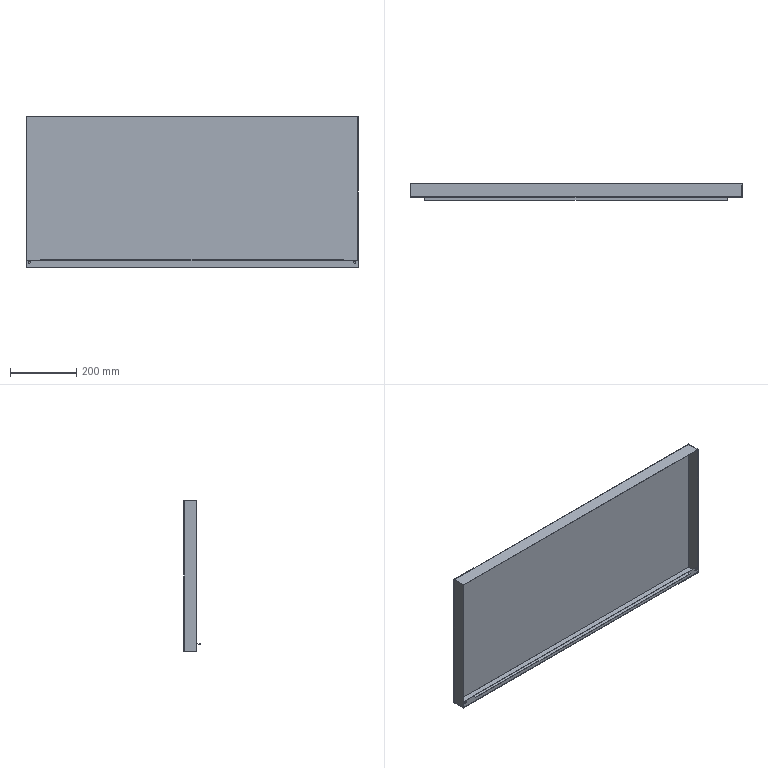Part | SolidWorks | features ICE 4, ExtruThin 1 | 1 solid | 23 faces | box 1002 x 50 x 455 mm | volume 600406 mm3 | plane 19 | cylinder 4 | commonest cylinder face diameters 5.5 x4
STEP:
#1=CARTESIAN_POINT('',(-491.,-39.,17.75));
#2=VERTEX_POINT('',#1);
#3=CARTESIAN_POINT('',(-491.,-39.,12.25));
#4=VERTEX_POINT('',#3);
#5=CARTESIAN_POINT('',(-491.,-39.,15.));
#6=DIRECTION('',(0.,-1.,0.));
#7=DIRECTION('',(0.,0.,-1.));
#8=AXIS2_PLACEMENT_3D('',#5,#6,#7);
#9=CIRCLE('',#8,2.75);
#10=EDGE_CURVE('',#2,#4,#9,.T.);
#11=ORIENTED_EDGE('',*,*,#10,.F.);
#12=CARTESIAN_POINT('',(-491.,-40.,17.75));
#13=VERTEX_POINT('',#12);
#14=CARTESIAN_POINT('',(-491.,-30.,17.75));
#15=DIRECTION('',(0.,-1.,0.));
#16=VECTOR('',#15,1000.);
#17=LINE('',#14,#16);
#18=EDGE_CURVE('',#2,#13,#17,.T.);
#19=ORIENTED_EDGE('',*,*,#18,.T.);
#20=CARTESIAN_POINT('',(-491.,-40.,12.25));
#21=VERTEX_POINT('',#20);
#22=CARTESIAN_POINT('',(-491.,-40.,15.));
#23=DIRECTION('',(0.,-1.,0.));
#24=DIRECTION('',(0.,0.,1.));
#25=AXIS2_PLACEMENT_3D('',#22,#23,#24);
#26=CIRCLE('',#25,2.75);
#27=EDGE_CURVE('',#13,#21,#26,.T.);
#28=ORIENTED_EDGE('',*,*,#27,.T.);
#29=CARTESIAN_POINT('',(-491.,-30.,12.25));
#30=DIRECTION('',(0.,-1.,0.));
#31=VECTOR('',#30,1000.);
#32=LINE('',#29,#31);
#33=EDGE_CURVE('',#4,#21,#32,.T.);
#34=ORIENTED_EDGE('',*,*,#33,.F.);
#35=EDGE_LOOP('',(#11,#19,#28,#34));
#36=FACE_OUTER_BOUND('',#35,.T.);
#37=CARTESIAN_POINT('',(-491.,-30.,15.));
#38=DIRECTION('',(0.,-1.,0.));
#39=DIRECTION('',(0.,0.,-1.));
#40=AXIS2_PLACEMENT_3D('',#37,#38,#39);
#41=CYLINDRICAL_SURFACE('',#40,2.75);
#42=ADVANCED_FACE('',(#36),#41,.F.);
#43=CARTESIAN_POINT('',(491.,-39.,17.75));
#44=VERTEX_POINT('',#43);
#45=CARTESIAN_POINT('',(491.,-39.,12.25));
#46=VERTEX_POINT('',#45);
#47=CARTESIAN_POINT('',(491.,-39.,15.));
#48=DIRECTION('',(0.,-1.,0.));
#49=DIRECTION('',(0.,0.,-1.));
#50=AXIS2_PLACEMENT_3D('',#47,#48,#49);
#51=CIRCLE('',#50,2.75);
#52=EDGE_CURVE('',#44,#46,#51,.T.);
#53=ORIENTED_EDGE('',*,*,#52,.F.);
#54=CARTESIAN_POINT('',(491.,-40.,17.75));
#55=VERTEX_POINT('',#54);
#56=CARTESIAN_POINT('',(491.,-30.,17.75));
#57=DIRECTION('',(0.,-1.,0.));
#58=VECTOR('',#57,1000.);
#59=LINE('',#56,#58);
#60=EDGE_CURVE('',#44,#55,#59,.T.);
#61=ORIENTED_EDGE('',*,*,#60,.T.);
#62=CARTESIAN_POINT('',(491.,-40.,12.25));
#63=VERTEX_POINT('',#62);
#64=CARTESIAN_POINT('',(491.,-40.,15.));
#65=DIRECTION('',(0.,-1.,0.));
#66=DIRECTION('',(0.,0.,-1.));
#67=AXIS2_PLACEMENT_3D('',#64,#65,#66);
#68=CIRCLE('',#67,2.75);
#69=EDGE_CURVE('',#55,#63,#68,.T.);
#70=ORIENTED_EDGE('',*,*,#69,.T.);
#71=CARTESIAN_POINT('',(491.,-30.,12.25));
#72=DIRECTION('',(0.,-1.,0.));
#73=VECTOR('',#72,1000.);
#74=LINE('',#71,#73);
#75=EDGE_CURVE('',#46,#63,#74,.T.);
#76=ORIENTED_EDGE('',*,*,#75,.F.);
#77=EDGE_LOOP('',(#53,#61,#70,#76));
#78=FACE_OUTER_BOUND('',#77,.T.);
#79=CARTESIAN_POINT('',(491.,-30.,15.));
#80=DIRECTION('',(0.,-1.,0.));
#81=DIRECTION('',(0.,0.,-1.));
#82=AXIS2_PLACEMENT_3D('',#79,#80,#81);
#83=CYLINDRICAL_SURFACE('',#82,2.75);
#84=ADVANCED_FACE('',(#78),#83,.F.);
#85=CARTESIAN_POINT('',(457.,-39.,23.));
#86=VERTEX_POINT('',#85);
#87=CARTESIAN_POINT('',(-457.,-39.,23.));
#88=VERTEX_POINT('',#87);
#89=CARTESIAN_POINT('',(500.,-39.,23.));
#90=DIRECTION('',(-1.,0.,0.));
#91=VECTOR('',#90,1000.);
#92=LINE('',#89,#91);
#93=EDGE_CURVE('',#86,#88,#92,.T.);
#94=ORIENTED_EDGE('',*,*,#93,.T.);
#95=CARTESIAN_POINT('',(-457.,-50.,23.));
#96=VERTEX_POINT('',#95);
#97=CARTESIAN_POINT('',(-457.,-30.,23.));
#98=DIRECTION('',(0.,-1.,0.));
#99=VECTOR('',#98,1000.);
#100=LINE('',#97,#99);
#101=EDGE_CURVE('',#88,#96,#100,.T.);
#102=ORIENTED_EDGE('',*,*,#101,.T.);
#103=CARTESIAN_POINT('',(457.,-50.,23.));
#104=VERTEX_POINT('',#103);
#105=CARTESIAN_POINT('',(500.,-50.,23.));
#106=DIRECTION('',(-1.,0.,0.));
#107=VECTOR('',#106,1000.);
#108=LINE('',#105,#107);
#109=EDGE_CURVE('',#104,#96,#108,.T.);
#110=ORIENTED_EDGE('',*,*,#109,.F.);
#111=CARTESIAN_POINT('',(457.,-30.,23.));
#112=DIRECTION('',(0.,-1.,0.));
#113=VECTOR('',#112,1000.);
#114=LINE('',#111,#113);
#115=EDGE_CURVE('',#86,#104,#114,.T.);
#116=ORIENTED_EDGE('',*,*,#115,.F.);
#117=EDGE_LOOP('',(#94,#102,#110,#116));
#118=FACE_OUTER_BOUND('',#117,.T.);
#119=CARTESIAN_POINT('',(500.,-40.,23.));
#120=DIRECTION('',(0.,0.,-1.));
#121=DIRECTION('',(-1.,0.,0.));
#122=AXIS2_PLACEMENT_3D('',#119,#120,#121);
#123=PLANE('',#122);
#124=ADVANCED_FACE('',(#118),#123,.F.);
#125=CARTESIAN_POINT('',(-457.,-50.,22.));
#126=VERTEX_POINT('',#125);
#127=CARTESIAN_POINT('',(-457.,-50.,22.));
#128=DIRECTION('',(0.,0.,1.));
#129=VECTOR('',#128,1000.);
#130=LINE('',#127,#129);
#131=EDGE_CURVE('',#126,#96,#130,.T.);
#132=ORIENTED_EDGE('',*,*,#131,.F.);
#133=CARTESIAN_POINT('',(457.,-50.,22.));
#134=VERTEX_POINT('',#133);
#135=CARTESIAN_POINT('',(500.,-50.,22.));
#136=DIRECTION('',(-1.,0.,0.));
#137=VECTOR('',#136,1000.);
#138=LINE('',#135,#137);
#139=EDGE_CURVE('',#134,#126,#138,.T.);
#140=ORIENTED_EDGE('',*,*,#139,.F.);
#141=CARTESIAN_POINT('',(457.,-50.,23.));
#142=DIRECTION('',(0.,0.,-1.));
#143=VECTOR('',#142,1000.);
#144=LINE('',#141,#143);
#145=EDGE_CURVE('',#104,#134,#144,.T.);
#146=ORIENTED_EDGE('',*,*,#145,.F.);
#147=ORIENTED_EDGE('',*,*,#109,.T.);
#148=EDGE_LOOP('',(#132,#140,#146,#147));
#149=FACE_OUTER_BOUND('',#148,.T.);
#150=CARTESIAN_POINT('',(500.,-50.,22.));
#151=DIRECTION('',(0.,-1.,0.));
#152=DIRECTION('',(0.,0.,-1.));
#153=AXIS2_PLACEMENT_3D('',#150,#151,#152);
#154=PLANE('',#153);
#155=ADVANCED_FACE('',(#149),#154,.T.);
#156=CARTESIAN_POINT('',(-457.,-40.,22.));
#157=VERTEX_POINT('',#156);
#158=CARTESIAN_POINT('',(-457.,-30.,22.));
#159=DIRECTION('',(0.,-1.,0.));
#160=VECTOR('',#159,1000.);
#161=LINE('',#158,#160);
#162=EDGE_CURVE('',#157,#126,#161,.T.);
#163=ORIENTED_EDGE('',*,*,#162,.F.);
#164=CARTESIAN_POINT('',(457.,-40.,22.));
#165=VERTEX_POINT('',#164);
#166=CARTESIAN_POINT('',(500.,-40.,22.));
#167=DIRECTION('',(-1.,0.,0.));
#168=VECTOR('',#167,1000.);
#169=LINE('',#166,#168);
#170=EDGE_CURVE('',#165,#157,#169,.T.);
#171=ORIENTED_EDGE('',*,*,#170,.F.);
#172=CARTESIAN_POINT('',(457.,-30.,22.));
#173=DIRECTION('',(0.,-1.,0.));
#174=VECTOR('',#173,1000.);
#175=LINE('',#172,#174);
#176=EDGE_CURVE('',#165,#134,#175,.T.);
#177=ORIENTED_EDGE('',*,*,#176,.T.);
#178=ORIENTED_EDGE('',*,*,#139,.T.);
#179=EDGE_LOOP('',(#163,#171,#177,#178));
#180=FACE_OUTER_BOUND('',#179,.T.);
#181=CARTESIAN_POINT('',(500.,-40.,22.));
#182=DIRECTION('',(0.,0.,-1.));
#183=DIRECTION('',(-1.,0.,0.));
#184=AXIS2_PLACEMENT_3D('',#181,#182,#183);
#185=PLANE('',#184);
#186=ADVANCED_FACE('',(#180),#185,.T.);
#187=CARTESIAN_POINT('',(501.,-40.,0.));
#188=VERTEX_POINT('',#187);
#189=CARTESIAN_POINT('',(-501.,-40.,0.));
#190=VERTEX_POINT('',#189);
#191=CARTESIAN_POINT('',(500.,-40.,0.));
#192=DIRECTION('',(-1.,0.,0.));
#193=VECTOR('',#192,1000.);
#194=LINE('',#191,#193);
#195=EDGE_CURVE('',#188,#190,#194,.T.);
#196=ORIENTED_EDGE('',*,*,#195,.T.);
#197=CARTESIAN_POINT('',(-501.,0.,0.));
#198=VERTEX_POINT('',#197);
#199=CARTESIAN_POINT('',(-501.,-40.,0.));
#200=DIRECTION('',(0.,-1.,0.));
#201=VECTOR('',#200,1000.);
#202=LINE('',#199,#201);
#203=EDGE_CURVE('',#198,#190,#202,.T.);
#204=ORIENTED_EDGE('',*,*,#203,.F.);
#205=CARTESIAN_POINT('',(501.,0.,0.));
#206=VERTEX_POINT('',#205);
#207=CARTESIAN_POINT('',(500.,0.,0.));
#208=DIRECTION('',(-1.,0.,0.));
#209=VECTOR('',#208,1000.);
#210=LINE('',#207,#209);
#211=EDGE_CURVE('',#206,#198,#210,.T.);
#212=ORIENTED_EDGE('',*,*,#211,.F.);
#213=CARTESIAN_POINT('',(501.,0.,0.));
#214=DIRECTION('',(0.,1.,0.));
#215=VECTOR('',#214,1000.);
#216=LINE('',#213,#215);
#217=EDGE_CURVE('',#188,#206,#216,.T.);
#218=ORIENTED_EDGE('',*,*,#217,.F.);
#219=EDGE_LOOP('',(#196,#204,#212,#218));
#220=FACE_OUTER_BOUND('',#219,.T.);
#221=CARTESIAN_POINT('',(500.,0.,0.));
#222=DIRECTION('',(0.,0.,-1.));
#223=DIRECTION('',(-1.,0.,0.));
#224=AXIS2_PLACEMENT_3D('',#221,#222,#223);
#225=PLANE('',#224);
#226=ADVANCED_FACE('',(#220),#225,.T.);
#227=ORIENTED_EDGE('',*,*,#211,.T.);
#228=CARTESIAN_POINT('',(-501.,0.,455.));
#229=VERTEX_POINT('',#228);
#230=CARTESIAN_POINT('',(-501.,0.,0.));
#231=DIRECTION('',(0.,0.,-1.));
#232=VECTOR('',#231,1000.);
#233=LINE('',#230,#232);
#234=EDGE_CURVE('',#229,#198,#233,.T.);
#235=ORIENTED_EDGE('',*,*,#234,.F.);
#236=CARTESIAN_POINT('',(501.,0.,455.));
#237=VERTEX_POINT('',#236);
#238=CARTESIAN_POINT('',(500.,0.,455.));
#239=DIRECTION('',(-1.,0.,0.));
#240=VECTOR('',#239,1000.);
#241=LINE('',#238,#240);
#242=EDGE_CURVE('',#237,#229,#241,.T.);
#243=ORIENTED_EDGE('',*,*,#242,.F.);
#244=CARTESIAN_POINT('',(501.,0.,455.));
#245=DIRECTION('',(0.,0.,1.));
#246=VECTOR('',#245,1000.);
#247=LINE('',#244,#246);
#248=EDGE_CURVE('',#206,#237,#247,.T.);
#249=ORIENTED_EDGE('',*,*,#248,.F.);
#250=EDGE_LOOP('',(#227,#235,#243,#249));
#251=FACE_OUTER_BOUND('',#250,.T.);
#252=CARTESIAN_POINT('',(500.,0.,0.));
#253=DIRECTION('',(0.,1.,0.));
#254=DIRECTION('',(0.,0.,1.));
#255=AXIS2_PLACEMENT_3D('',#252,#253,#254);
#256=PLANE('',#255);
#257=ADVANCED_FACE('',(#251),#256,.T.);
#258=ORIENTED_EDGE('',*,*,#242,.T.);
#259=CARTESIAN_POINT('',(-501.,-40.,455.));
#260=VERTEX_POINT('',#259);
#261=CARTESIAN_POINT('',(-501.,0.,455.));
#262=DIRECTION('',(0.,1.,0.));
#263=VECTOR('',#262,1000.);
#264=LINE('',#261,#263);
#265=EDGE_CURVE('',#260,#229,#264,.T.);
#266=ORIENTED_EDGE('',*,*,#265,.F.);
#267=CARTESIAN_POINT('',(501.,-40.,455.));
#268=VERTEX_POINT('',#267);
#269=CARTESIAN_POINT('',(500.,-40.,455.));
#270=DIRECTION('',(-1.,0.,0.));
#271=VECTOR('',#270,1000.);
#272=LINE('',#269,#271);
#273=EDGE_CURVE('',#268,#260,#272,.T.);
#274=ORIENTED_EDGE('',*,*,#273,.F.);
#275=CARTESIAN_POINT('',(501.,-40.,455.));
#276=DIRECTION('',(0.,-1.,0.));
#277=VECTOR('',#276,1000.);
#278=LINE('',#275,#277);
#279=EDGE_CURVE('',#237,#268,#278,.T.);
#280=ORIENTED_EDGE('',*,*,#279,.F.);
#281=EDGE_LOOP('',(#258,#266,#274,#280));
#282=FACE_OUTER_BOUND('',#281,.T.);
#283=CARTESIAN_POINT('',(500.,0.,455.));
#284=DIRECTION('',(0.,0.,1.));
#285=DIRECTION('',(1.,0.,0.));
#286=AXIS2_PLACEMENT_3D('',#283,#284,#285);
#287=PLANE('',#286);
#288=ADVANCED_FACE('',(#282),#287,.T.);
#289=CARTESIAN_POINT('',(-491.,-40.,15.));
#290=DIRECTION('',(0.,-1.,0.));
#291=DIRECTION('',(0.,0.,1.));
#292=AXIS2_PLACEMENT_3D('',#289,#290,#291);
#293=CIRCLE('',#292,2.75);
#294=EDGE_CURVE('',#21,#13,#293,.T.);
#295=ORIENTED_EDGE('',*,*,#294,.F.);
#296=ORIENTED_EDGE('',*,*,#27,.F.);
#297=EDGE_LOOP('',(#295,#296));
#298=FACE_BOUND('',#297,.T.);
#299=CARTESIAN_POINT('',(491.,-40.,15.));
#300=DIRECTION('',(0.,-1.,0.));
#301=DIRECTION('',(0.,0.,-1.));
#302=AXIS2_PLACEMENT_3D('',#299,#300,#301);
#303=CIRCLE('',#302,2.75);
#304=EDGE_CURVE('',#63,#55,#303,.T.);
#305=ORIENTED_EDGE('',*,*,#304,.F.);
#306=ORIENTED_EDGE('',*,*,#69,.F.);
#307=EDGE_LOOP('',(#305,#306));
#308=FACE_BOUND('',#307,.T.);
#309=CARTESIAN_POINT('',(500.,-40.,22.));
#310=VERTEX_POINT('',#309);
#311=CARTESIAN_POINT('',(500.,-40.,22.));
#312=DIRECTION('',(-1.,0.,0.));
#313=VECTOR('',#312,1000.);
#314=LINE('',#311,#313);
#315=EDGE_CURVE('',#310,#165,#314,.T.);
#316=ORIENTED_EDGE('',*,*,#315,.T.);
#317=ORIENTED_EDGE('',*,*,#170,.T.);
#318=CARTESIAN_POINT('',(-500.,-40.,22.));
#319=VERTEX_POINT('',#318);
#320=CARTESIAN_POINT('',(500.,-40.,22.));
#321=DIRECTION('',(1.,0.,0.));
#322=VECTOR('',#321,1000.);
#323=LINE('',#320,#322);
#324=EDGE_CURVE('',#319,#157,#323,.T.);
#325=ORIENTED_EDGE('',*,*,#324,.F.);
#326=CARTESIAN_POINT('',(-500.,-40.,454.));
#327=VERTEX_POINT('',#326);
#328=CARTESIAN_POINT('',(-500.,-40.,455.));
#329=DIRECTION('',(0.,0.,1.));
#330=VECTOR('',#329,1000.);
#331=LINE('',#328,#330);
#332=EDGE_CURVE('',#319,#327,#331,.T.);
#333=ORIENTED_EDGE('',*,*,#332,.T.);
#334=CARTESIAN_POINT('',(500.,-40.,454.));
#335=VERTEX_POINT('',#334);
#336=CARTESIAN_POINT('',(500.,-40.,454.));
#337=DIRECTION('',(-1.,0.,0.));
#338=VECTOR('',#337,1000.);
#339=LINE('',#336,#338);
#340=EDGE_CURVE('',#335,#327,#339,.T.);
#341=ORIENTED_EDGE('',*,*,#340,.F.);
#342=CARTESIAN_POINT('',(500.,-40.,0.));
#343=DIRECTION('',(0.,0.,-1.));
#344=VECTOR('',#343,1000.);
#345=LINE('',#342,#344);
#346=EDGE_CURVE('',#335,#310,#345,.T.);
#347=ORIENTED_EDGE('',*,*,#346,.T.);
#348=EDGE_LOOP('',(#316,#317,#325,#333,#341,#347));
#349=FACE_BOUND('',#348,.T.);
#350=ORIENTED_EDGE('',*,*,#273,.T.);
#351=CARTESIAN_POINT('',(-501.,-40.,455.));
#352=DIRECTION('',(0.,0.,1.));
#353=VECTOR('',#352,1000.);
#354=LINE('',#351,#353);
#355=EDGE_CURVE('',#190,#260,#354,.T.);
#356=ORIENTED_EDGE('',*,*,#355,.F.);
#357=ORIENTED_EDGE('',*,*,#195,.F.);
#358=CARTESIAN_POINT('',(501.,-40.,0.));
#359=DIRECTION('',(0.,0.,-1.));
#360=VECTOR('',#359,1000.);
#361=LINE('',#358,#360);
#362=EDGE_CURVE('',#268,#188,#361,.T.);
#363=ORIENTED_EDGE('',*,*,#362,.F.);
#364=EDGE_LOOP('',(#350,#356,#357,#363));
#365=FACE_OUTER_BOUND('',#364,.T.);
#366=CARTESIAN_POINT('',(500.,-40.,454.));
#367=DIRECTION('',(0.,-1.,0.));
#368=DIRECTION('',(0.,0.,-1.));
#369=AXIS2_PLACEMENT_3D('',#366,#367,#368);
#370=PLANE('',#369);
#371=ADVANCED_FACE('',(#298,#308,#349,#365),#370,.T.);
#372=CARTESIAN_POINT('',(-500.,-1.,454.));
#373=VERTEX_POINT('',#372);
#374=CARTESIAN_POINT('',(-500.,0.,454.));
#375=DIRECTION('',(0.,1.,0.));
#376=VECTOR('',#375,1000.);
#377=LINE('',#374,#376);
#378=EDGE_CURVE('',#327,#373,#377,.T.);
#379=ORIENTED_EDGE('',*,*,#378,.T.);
#380=CARTESIAN_POINT('',(500.,-1.,454.));
#381=VERTEX_POINT('',#380);
#382=CARTESIAN_POINT('',(500.,-1.,454.));
#383=DIRECTION('',(-1.,0.,0.));
#384=VECTOR('',#383,1000.);
#385=LINE('',#382,#384);
#386=EDGE_CURVE('',#381,#373,#385,.T.);
#387=ORIENTED_EDGE('',*,*,#386,.F.);
#388=CARTESIAN_POINT('',(500.,0.,454.));
#389=DIRECTION('',(0.,1.,0.));
#390=VECTOR('',#389,1000.);
#391=LINE('',#388,#390);
#392=EDGE_CURVE('',#335,#381,#391,.T.);
#393=ORIENTED_EDGE('',*,*,#392,.F.);
#394=ORIENTED_EDGE('',*,*,#340,.T.);
#395=EDGE_LOOP('',(#379,#387,#393,#394));
#396=FACE_OUTER_BOUND('',#395,.T.);
#397=CARTESIAN_POINT('',(500.,0.,454.));
#398=DIRECTION('',(0.,0.,1.));
#399=DIRECTION('',(1.,0.,0.));
#400=AXIS2_PLACEMENT_3D('',#397,#398,#399);
#401=PLANE('',#400);
#402=ADVANCED_FACE('',(#396),#401,.F.);
#403=CARTESIAN_POINT('',(-500.,-1.,1.));
#404=VERTEX_POINT('',#403);
#405=CARTESIAN_POINT('',(-500.,-1.,0.));
#406=DIRECTION('',(0.,0.,-1.));
#407=VECTOR('',#406,1000.);
#408=LINE('',#405,#407);
#409=EDGE_CURVE('',#373,#404,#408,.T.);
#410=ORIENTED_EDGE('',*,*,#409,.T.);
#411=CARTESIAN_POINT('',(500.,-1.,1.));
#412=VERTEX_POINT('',#411);
#413=CARTESIAN_POINT('',(500.,-1.,1.));
#414=DIRECTION('',(-1.,0.,0.));
#415=VECTOR('',#414,1000.);
#416=LINE('',#413,#415);
#417=EDGE_CURVE('',#412,#404,#416,.T.);
#418=ORIENTED_EDGE('',*,*,#417,.F.);
#419=CARTESIAN_POINT('',(500.,-1.,0.));
#420=DIRECTION('',(0.,0.,-1.));
#421=VECTOR('',#420,1000.);
#422=LINE('',#419,#421);
#423=EDGE_CURVE('',#381,#412,#422,.T.);
#424=ORIENTED_EDGE('',*,*,#423,.F.);
#425=ORIENTED_EDGE('',*,*,#386,.T.);
#426=EDGE_LOOP('',(#410,#418,#424,#425));
#427=FACE_OUTER_BOUND('',#426,.T.);
#428=CARTESIAN_POINT('',(500.,-1.,0.));
#429=DIRECTION('',(0.,1.,0.));
#430=DIRECTION('',(0.,0.,1.));
#431=AXIS2_PLACEMENT_3D('',#428,#429,#430);
#432=PLANE('',#431);
#433=ADVANCED_FACE('',(#427),#432,.F.);
#434=CARTESIAN_POINT('',(-500.,-39.,1.));
#435=VERTEX_POINT('',#434);
#436=CARTESIAN_POINT('',(-500.,0.,1.));
#437=DIRECTION('',(0.,-1.,0.));
#438=VECTOR('',#437,1000.);
#439=LINE('',#436,#438);
#440=EDGE_CURVE('',#404,#435,#439,.T.);
#441=ORIENTED_EDGE('',*,*,#440,.T.);
#442=CARTESIAN_POINT('',(500.,-39.,1.));
#443=VERTEX_POINT('',#442);
#444=CARTESIAN_POINT('',(500.,-39.,1.));
#445=DIRECTION('',(-1.,0.,0.));
#446=VECTOR('',#445,1000.);
#447=LINE('',#444,#446);
#448=EDGE_CURVE('',#443,#435,#447,.T.);
#449=ORIENTED_EDGE('',*,*,#448,.F.);
#450=CARTESIAN_POINT('',(500.,0.,1.));
#451=DIRECTION('',(0.,-1.,0.));
#452=VECTOR('',#451,1000.);
#453=LINE('',#450,#452);
#454=EDGE_CURVE('',#412,#443,#453,.T.);
#455=ORIENTED_EDGE('',*,*,#454,.F.);
#456=ORIENTED_EDGE('',*,*,#417,.T.);
#457=EDGE_LOOP('',(#441,#449,#455,#456));
#458=FACE_OUTER_BOUND('',#457,.T.);
#459=CARTESIAN_POINT('',(500.,0.,1.));
#460=DIRECTION('',(0.,0.,-1.));
#461=DIRECTION('',(-1.,0.,0.));
#462=AXIS2_PLACEMENT_3D('',#459,#460,#461);
#463=PLANE('',#462);
#464=ADVANCED_FACE('',(#458),#463,.F.);
#465=CARTESIAN_POINT('',(-491.,-39.,15.));
#466=DIRECTION('',(0.,-1.,0.));
#467=DIRECTION('',(0.,0.,-1.));
#468=AXIS2_PLACEMENT_3D('',#465,#466,#467);
#469=CIRCLE('',#468,2.75);
#470=EDGE_CURVE('',#4,#2,#469,.T.);
#471=ORIENTED_EDGE('',*,*,#470,.T.);
#472=ORIENTED_EDGE('',*,*,#10,.T.);
#473=EDGE_LOOP('',(#471,#472));
#474=FACE_BOUND('',#473,.T.);
#475=CARTESIAN_POINT('',(491.,-39.,15.));
#476=DIRECTION('',(0.,-1.,0.));
#477=DIRECTION('',(0.,0.,-1.));
#478=AXIS2_PLACEMENT_3D('',#475,#476,#477);
#479=CIRCLE('',#478,2.75);
#480=EDGE_CURVE('',#46,#44,#479,.T.);
#481=ORIENTED_EDGE('',*,*,#480,.T.);
#482=ORIENTED_EDGE('',*,*,#52,.T.);
#483=EDGE_LOOP('',(#481,#482));
#484=FACE_BOUND('',#483,.T.);
#485=CARTESIAN_POINT('',(-500.,-39.,22.));
#486=VERTEX_POINT('',#485);
#487=CARTESIAN_POINT('',(-457.,-39.,22.));
#488=VERTEX_POINT('',#487);
#489=CARTESIAN_POINT('',(500.,-39.,22.));
#490=DIRECTION('',(1.,0.,0.));
#491=VECTOR('',#490,1000.);
#492=LINE('',#489,#491);
#493=EDGE_CURVE('',#486,#488,#492,.T.);
#494=ORIENTED_EDGE('',*,*,#493,.T.);
#495=CARTESIAN_POINT('',(-457.,-39.,0.));
#496=DIRECTION('',(0.,0.,1.));
#497=VECTOR('',#496,1000.);
#498=LINE('',#495,#497);
#499=EDGE_CURVE('',#488,#88,#498,.T.);
#500=ORIENTED_EDGE('',*,*,#499,.T.);
#501=ORIENTED_EDGE('',*,*,#93,.F.);
#502=CARTESIAN_POINT('',(457.,-39.,22.));
#503=VERTEX_POINT('',#502);
#504=CARTESIAN_POINT('',(457.,-39.,0.));
#505=DIRECTION('',(0.,0.,-1.));
#506=VECTOR('',#505,1000.);
#507=LINE('',#504,#506);
#508=EDGE_CURVE('',#86,#503,#507,.T.);
#509=ORIENTED_EDGE('',*,*,#508,.T.);
#510=CARTESIAN_POINT('',(500.,-39.,22.));
#511=VERTEX_POINT('',#510);
#512=CARTESIAN_POINT('',(500.,-39.,22.));
#513=DIRECTION('',(1.,0.,0.));
#514=VECTOR('',#513,1000.);
#515=LINE('',#512,#514);
#516=EDGE_CURVE('',#503,#511,#515,.T.);
#517=ORIENTED_EDGE('',*,*,#516,.T.);
#518=CARTESIAN_POINT('',(500.,-39.,0.));
#519=DIRECTION('',(0.,0.,1.));
#520=VECTOR('',#519,1000.);
#521=LINE('',#518,#520);
#522=EDGE_CURVE('',#443,#511,#521,.T.);
#523=ORIENTED_EDGE('',*,*,#522,.F.);
#524=ORIENTED_EDGE('',*,*,#448,.T.);
#525=CARTESIAN_POINT('',(-500.,-39.,0.));
#526=DIRECTION('',(0.,0.,1.));
#527=VECTOR('',#526,1000.);
#528=LINE('',#525,#527);
#529=EDGE_CURVE('',#435,#486,#528,.T.);
#530=ORIENTED_EDGE('',*,*,#529,.T.);
#531=EDGE_LOOP('',(#494,#500,#501,#509,#517,#523,#524,#530));
#532=FACE_OUTER_BOUND('',#531,.T.);
#533=CARTESIAN_POINT('',(500.,-39.,0.));
#534=DIRECTION('',(0.,-1.,0.));
#535=DIRECTION('',(0.,0.,-1.));
#536=AXIS2_PLACEMENT_3D('',#533,#534,#535);
#537=PLANE('',#536);
#538=ADVANCED_FACE('',(#474,#484,#532),#537,.F.);
#539=ORIENTED_EDGE('',*,*,#362,.T.);
#540=ORIENTED_EDGE('',*,*,#217,.T.);
#541=ORIENTED_EDGE('',*,*,#248,.T.);
#542=ORIENTED_EDGE('',*,*,#279,.T.);
#543=EDGE_LOOP('',(#539,#540,#541,#542));
#544=FACE_OUTER_BOUND('',#543,.T.);
#545=CARTESIAN_POINT('',(501.,-40.,455.));
#546=DIRECTION('',(-1.,0.,0.));
#547=DIRECTION('',(0.,0.,1.));
#548=AXIS2_PLACEMENT_3D('',#545,#546,#547);
#549=PLANE('',#548);
#550=ADVANCED_FACE('',(#544),#549,.F.);
#551=ORIENTED_EDGE('',*,*,#522,.T.);
#552=CARTESIAN_POINT('',(500.,-30.,22.));
#553=DIRECTION('',(0.,-1.,0.));
#554=VECTOR('',#553,1000.);
#555=LINE('',#552,#554);
#556=EDGE_CURVE('',#511,#310,#555,.T.);
#557=ORIENTED_EDGE('',*,*,#556,.T.);
#558=ORIENTED_EDGE('',*,*,#346,.F.);
#559=ORIENTED_EDGE('',*,*,#392,.T.);
#560=ORIENTED_EDGE('',*,*,#423,.T.);
#561=ORIENTED_EDGE('',*,*,#454,.T.);
#562=EDGE_LOOP('',(#551,#557,#558,#559,#560,#561));
#563=FACE_OUTER_BOUND('',#562,.T.);
#564=CARTESIAN_POINT('',(500.,-40.,455.));
#565=DIRECTION('',(-1.,0.,0.));
#566=DIRECTION('',(0.,0.,1.));
#567=AXIS2_PLACEMENT_3D('',#564,#565,#566);
#568=PLANE('',#567);
#569=ADVANCED_FACE('',(#563),#568,.T.);
#570=CARTESIAN_POINT('',(-500.,-30.,22.));
#571=DIRECTION('',(0.,-1.,0.));
#572=VECTOR('',#571,1000.);
#573=LINE('',#570,#572);
#574=EDGE_CURVE('',#486,#319,#573,.T.);
#575=ORIENTED_EDGE('',*,*,#574,.F.);
#576=ORIENTED_EDGE('',*,*,#529,.F.);
#577=ORIENTED_EDGE('',*,*,#440,.F.);
#578=ORIENTED_EDGE('',*,*,#409,.F.);
#579=ORIENTED_EDGE('',*,*,#378,.F.);
#580=ORIENTED_EDGE('',*,*,#332,.F.);
#581=EDGE_LOOP('',(#575,#576,#577,#578,#579,#580));
#582=FACE_OUTER_BOUND('',#581,.T.);
#583=CARTESIAN_POINT('',(-500.,-40.,0.));
#584=DIRECTION('',(1.,0.,0.));
#585=DIRECTION('',(0.,0.,-1.));
#586=AXIS2_PLACEMENT_3D('',#583,#584,#585);
#587=PLANE('',#586);
#588=ADVANCED_FACE('',(#582),#587,.T.);
#589=ORIENTED_EDGE('',*,*,#355,.T.);
#590=ORIENTED_EDGE('',*,*,#265,.T.);
#591=ORIENTED_EDGE('',*,*,#234,.T.);
#592=ORIENTED_EDGE('',*,*,#203,.T.);
#593=EDGE_LOOP('',(#589,#590,#591,#592));
#594=FACE_OUTER_BOUND('',#593,.T.);
#595=CARTESIAN_POINT('',(-501.,-40.,0.));
#596=DIRECTION('',(1.,0.,0.));
#597=DIRECTION('',(0.,0.,-1.));
#598=AXIS2_PLACEMENT_3D('',#595,#596,#597);
#599=PLANE('',#598);
#600=ADVANCED_FACE('',(#594),#599,.F.);
#601=ORIENTED_EDGE('',*,*,#115,.T.);
#602=ORIENTED_EDGE('',*,*,#145,.T.);
#603=ORIENTED_EDGE('',*,*,#176,.F.);
#604=CARTESIAN_POINT('',(457.,-30.,22.));
#605=DIRECTION('',(0.,-1.,0.));
#606=VECTOR('',#605,1000.);
#607=LINE('',#604,#606);
#608=EDGE_CURVE('',#503,#165,#607,.T.);
#609=ORIENTED_EDGE('',*,*,#608,.F.);
#610=ORIENTED_EDGE('',*,*,#508,.F.);
#611=EDGE_LOOP('',(#601,#602,#603,#609,#610));
#612=FACE_OUTER_BOUND('',#611,.T.);
#613=CARTESIAN_POINT('',(457.,-30.,23.));
#614=DIRECTION('',(-1.,0.,0.));
#615=DIRECTION('',(0.,0.,1.));
#616=AXIS2_PLACEMENT_3D('',#613,#614,#615);
#617=PLANE('',#616);
#618=ADVANCED_FACE('',(#612),#617,.F.);
#619=ORIENTED_EDGE('',*,*,#315,.F.);
#620=ORIENTED_EDGE('',*,*,#556,.F.);
#621=ORIENTED_EDGE('',*,*,#516,.F.);
#622=ORIENTED_EDGE('',*,*,#608,.T.);
#623=EDGE_LOOP('',(#619,#620,#621,#622));
#624=FACE_OUTER_BOUND('',#623,.T.);
#625=CARTESIAN_POINT('',(500.,-30.,22.));
#626=DIRECTION('',(0.,0.,-1.));
#627=DIRECTION('',(-1.,0.,0.));
#628=AXIS2_PLACEMENT_3D('',#625,#626,#627);
#629=PLANE('',#628);
#630=ADVANCED_FACE('',(#624),#629,.F.);
#631=CARTESIAN_POINT('',(-457.,-30.,22.));
#632=DIRECTION('',(0.,-1.,0.));
#633=VECTOR('',#632,1000.);
#634=LINE('',#631,#633);
#635=EDGE_CURVE('',#488,#157,#634,.T.);
#636=ORIENTED_EDGE('',*,*,#635,.T.);
#637=ORIENTED_EDGE('',*,*,#162,.T.);
#638=ORIENTED_EDGE('',*,*,#131,.T.);
#639=ORIENTED_EDGE('',*,*,#101,.F.);
#640=ORIENTED_EDGE('',*,*,#499,.F.);
#641=EDGE_LOOP('',(#636,#637,#638,#639,#640));
#642=FACE_OUTER_BOUND('',#641,.T.);
#643=CARTESIAN_POINT('',(-457.,-30.,22.));
#644=DIRECTION('',(1.,0.,0.));
#645=DIRECTION('',(0.,0.,-1.));
#646=AXIS2_PLACEMENT_3D('',#643,#644,#645);
#647=PLANE('',#646);
#648=ADVANCED_FACE('',(#642),#647,.F.);
#649=ORIENTED_EDGE('',*,*,#324,.T.);
#650=ORIENTED_EDGE('',*,*,#635,.F.);
#651=ORIENTED_EDGE('',*,*,#493,.F.);
#652=ORIENTED_EDGE('',*,*,#574,.T.);
#653=EDGE_LOOP('',(#649,#650,#651,#652));
#654=FACE_OUTER_BOUND('',#653,.T.);
#655=CARTESIAN_POINT('',(-500.,-30.,22.));
#656=DIRECTION('',(0.,0.,-1.));
#657=DIRECTION('',(-1.,0.,0.));
#658=AXIS2_PLACEMENT_3D('',#655,#656,#657);
#659=PLANE('',#658);
#660=ADVANCED_FACE('',(#654),#659,.F.);
#661=ORIENTED_EDGE('',*,*,#60,.F.);
#662=ORIENTED_EDGE('',*,*,#480,.F.);
#663=ORIENTED_EDGE('',*,*,#75,.T.);
#664=ORIENTED_EDGE('',*,*,#304,.T.);
#665=EDGE_LOOP('',(#661,#662,#663,#664));
#666=FACE_OUTER_BOUND('',#665,.T.);
#667=CARTESIAN_POINT('',(491.,-30.,15.));
#668=DIRECTION('',(0.,-1.,0.));
#669=DIRECTION('',(0.,0.,-1.));
#670=AXIS2_PLACEMENT_3D('',#667,#668,#669);
#671=CYLINDRICAL_SURFACE('',#670,2.75);
#672=ADVANCED_FACE('',(#666),#671,.F.);
#673=ORIENTED_EDGE('',*,*,#18,.F.);
#674=ORIENTED_EDGE('',*,*,#470,.F.);
#675=ORIENTED_EDGE('',*,*,#33,.T.);
#676=ORIENTED_EDGE('',*,*,#294,.T.);
#677=EDGE_LOOP('',(#673,#674,#675,#676));
#678=FACE_OUTER_BOUND('',#677,.T.);
#679=CARTESIAN_POINT('',(-491.,-30.,15.));
#680=DIRECTION('',(0.,-1.,0.));
#681=DIRECTION('',(0.,0.,-1.));
#682=AXIS2_PLACEMENT_3D('',#679,#680,#681);
#683=CYLINDRICAL_SURFACE('',#682,2.75);
#684=ADVANCED_FACE('',(#678),#683,.F.);
#685=CLOSED_SHELL('',(#42,#84,#124,#155,#186,#226,#257,#288,#371,#402,#433,#464,#538,#550,#569,#588,#600,#618,#630,#648,#660,#672,#684));
#686=MANIFOLD_SOLID_BREP('',#685);
#687=CARTESIAN_POINT('',(0.,0.,0.));
#688=DIRECTION('',(0.,0.,1.));
#689=DIRECTION('',(1.,0.,0.));
#690=AXIS2_PLACEMENT_3D('',#687,#688,#689);
#691=(LENGTH_UNIT()NAMED_UNIT(*)SI_UNIT(.MILLI.,.METRE.));
#692=UNCERTAINTY_MEASURE_WITH_UNIT(LENGTH_MEASURE(0.00001),#691,'','');
#693=(NAMED_UNIT(*)PLANE_ANGLE_UNIT()SI_UNIT($,.RADIAN.));
#694=(NAMED_UNIT(*)SI_UNIT($,.STERADIAN.)SOLID_ANGLE_UNIT());
#695=(GEOMETRIC_REPRESENTATION_CONTEXT(3)GLOBAL_UNCERTAINTY_ASSIGNED_CONTEXT((#692))GLOBAL_UNIT_ASSIGNED_CONTEXT((#691,#693,#694))REPRESENTATION_CONTEXT('',''));
#696=ADVANCED_BREP_SHAPE_REPRESENTATION('',(#686,#690),#695);